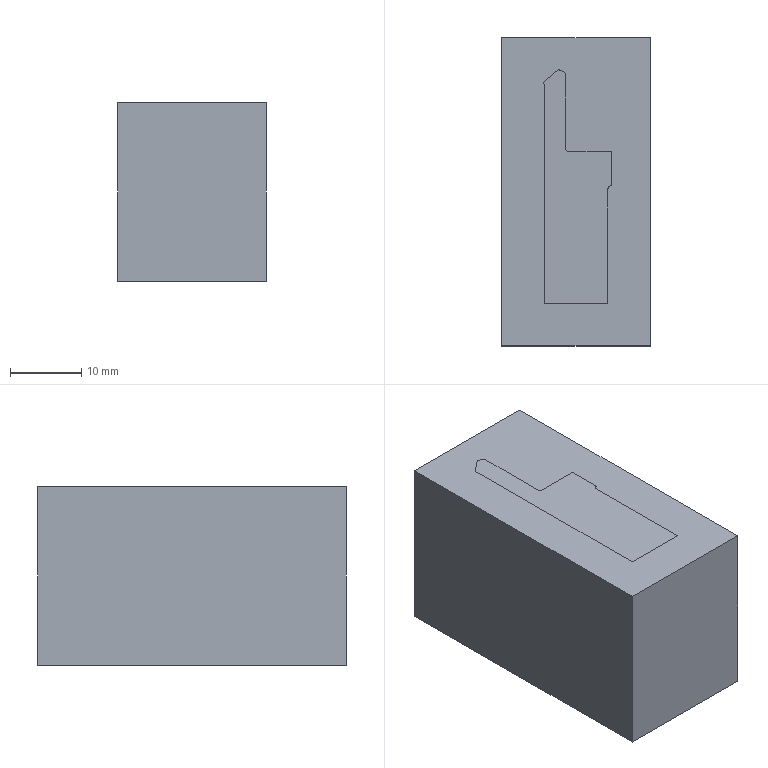Part | NX | features BREP 2 | 2 solids | 24 faces | box 20.877 x 43.224 x 25 mm | volume 39456 mm3 | plane 19 | cylinder 5 | commonest cylinder face diameters 0.9 x4 1.1 x1
STEP:
#1=CARTESIAN_POINT('',(-10.633,-22.355,-25.6));
#2=VERTEX_POINT('',#1);
#3=CARTESIAN_POINT('',(-10.633,20.868,-25.6));
#4=VERTEX_POINT('',#3);
#5=CARTESIAN_POINT('',(-10.633,-22.355,-25.6));
#6=DIRECTION('',(0.,1.,0.));
#7=VECTOR('',#6,1000.);
#8=LINE('',#5,#7);
#9=EDGE_CURVE('',#2,#4,#8,.T.);
#10=ORIENTED_EDGE('',*,*,#9,.T.);
#11=CARTESIAN_POINT('',(10.243,20.868,-25.6));
#12=VERTEX_POINT('',#11);
#13=CARTESIAN_POINT('',(-10.633,20.868,-25.6));
#14=DIRECTION('',(1.,0.,0.));
#15=VECTOR('',#14,1000.);
#16=LINE('',#13,#15);
#17=EDGE_CURVE('',#4,#12,#16,.T.);
#18=ORIENTED_EDGE('',*,*,#17,.T.);
#19=CARTESIAN_POINT('',(10.243,-22.355,-25.6));
#20=VERTEX_POINT('',#19);
#21=CARTESIAN_POINT('',(10.243,20.868,-25.6));
#22=DIRECTION('',(0.,-1.,0.));
#23=VECTOR('',#22,1000.);
#24=LINE('',#21,#23);
#25=EDGE_CURVE('',#12,#20,#24,.T.);
#26=ORIENTED_EDGE('',*,*,#25,.T.);
#27=CARTESIAN_POINT('',(10.243,-22.355,-25.6));
#28=DIRECTION('',(-1.,0.,0.));
#29=VECTOR('',#28,1000.);
#30=LINE('',#27,#29);
#31=EDGE_CURVE('',#20,#2,#30,.T.);
#32=ORIENTED_EDGE('',*,*,#31,.T.);
#33=EDGE_LOOP('',(#10,#18,#26,#32));
#34=FACE_BOUND('',#33,.T.);
#35=CARTESIAN_POINT('',(4.293,-0.3316,-25.6));
#36=VERTEX_POINT('',#35);
#37=CARTESIAN_POINT('',(4.793,0.1156,-25.6));
#38=VERTEX_POINT('',#37);
#39=CARTESIAN_POINT('',(4.743,-0.3316,-25.6));
#40=DIRECTION('',(0.,0.,-1.));
#41=DIRECTION('',(1.,0.,0.));
#42=AXIS2_PLACEMENT_3D('',#39,#40,#41);
#43=CIRCLE('',#42,0.45);
#44=EDGE_CURVE('',#36,#38,#43,.T.);
#45=ORIENTED_EDGE('',*,*,#44,.T.);
#46=CARTESIAN_POINT('',(4.793,4.918,-25.6));
#47=VERTEX_POINT('',#46);
#48=CARTESIAN_POINT('',(4.793,10.146,-25.6));
#49=DIRECTION('',(0.,1.,0.));
#50=VECTOR('',#49,1000.);
#51=LINE('',#48,#50);
#52=EDGE_CURVE('',#38,#47,#51,.T.);
#53=ORIENTED_EDGE('',*,*,#52,.T.);
#54=CARTESIAN_POINT('',(-1.233,4.918,-25.6));
#55=VERTEX_POINT('',#54);
#56=CARTESIAN_POINT('',(13.817,4.918,-25.6));
#57=DIRECTION('',(-1.,0.,0.));
#58=VECTOR('',#57,1000.);
#59=LINE('',#56,#58);
#60=EDGE_CURVE('',#47,#55,#59,.T.);
#61=ORIENTED_EDGE('',*,*,#60,.T.);
#62=CARTESIAN_POINT('',(-1.683,5.368,-25.6));
#63=VERTEX_POINT('',#62);
#64=CARTESIAN_POINT('',(-1.233,5.368,-25.6));
#65=DIRECTION('',(0.,0.,-1.));
#66=DIRECTION('',(1.,0.,0.));
#67=AXIS2_PLACEMENT_3D('',#64,#65,#66);
#68=CIRCLE('',#67,0.45);
#69=EDGE_CURVE('',#55,#63,#68,.T.);
#70=ORIENTED_EDGE('',*,*,#69,.T.);
#71=CARTESIAN_POINT('',(-1.683,15.668,-25.6));
#72=VERTEX_POINT('',#71);
#73=CARTESIAN_POINT('',(-1.683,10.146,-25.6));
#74=DIRECTION('',(0.,1.,0.));
#75=VECTOR('',#74,1000.);
#76=LINE('',#73,#75);
#77=EDGE_CURVE('',#63,#72,#76,.T.);
#78=ORIENTED_EDGE('',*,*,#77,.T.);
#79=CARTESIAN_POINT('',(-2.233,16.218,-25.6));
#80=VERTEX_POINT('',#79);
#81=CARTESIAN_POINT('',(-2.233,15.668,-25.6));
#82=DIRECTION('',(0.,0.,1.));
#83=DIRECTION('',(1.,0.,0.));
#84=AXIS2_PLACEMENT_3D('',#81,#82,#83);
#85=CIRCLE('',#84,0.55);
#86=EDGE_CURVE('',#72,#80,#85,.T.);
#87=ORIENTED_EDGE('',*,*,#86,.T.);
#88=CARTESIAN_POINT('',(-2.613,16.427,-25.6));
#89=VERTEX_POINT('',#88);
#90=CARTESIAN_POINT('',(-2.233,16.668,-25.6));
#91=DIRECTION('',(0.,0.,-1.));
#92=DIRECTION('',(1.,0.,0.));
#93=AXIS2_PLACEMENT_3D('',#90,#91,#92);
#94=CIRCLE('',#93,0.45);
#95=EDGE_CURVE('',#80,#89,#94,.T.);
#96=ORIENTED_EDGE('',*,*,#95,.T.);
#97=CARTESIAN_POINT('',(-4.816,14.657,-25.6));
#98=VERTEX_POINT('',#97);
#99=CARTESIAN_POINT('',(-5.164,14.377,-25.6));
#100=DIRECTION('',(-0.7795,-0.6264,0.));
#101=VECTOR('',#100,1000.);
#102=LINE('',#99,#101);
#103=EDGE_CURVE('',#89,#98,#102,.T.);
#104=ORIENTED_EDGE('',*,*,#103,.T.);
#105=CARTESIAN_POINT('',(-4.683,14.338,-25.6));
#106=VERTEX_POINT('',#105);
#107=CARTESIAN_POINT('',(-5.133,14.338,-25.6));
#108=DIRECTION('',(0.,0.,-1.));
#109=DIRECTION('',(1.,0.,0.));
#110=AXIS2_PLACEMENT_3D('',#107,#108,#109);
#111=CIRCLE('',#110,0.45);
#112=EDGE_CURVE('',#98,#106,#111,.T.);
#113=ORIENTED_EDGE('',*,*,#112,.T.);
#114=CARTESIAN_POINT('',(-4.683,-16.405,-25.6));
#115=VERTEX_POINT('',#114);
#116=CARTESIAN_POINT('',(-4.683,10.146,-25.6));
#117=DIRECTION('',(0.,-1.,0.));
#118=VECTOR('',#117,1000.);
#119=LINE('',#116,#118);
#120=EDGE_CURVE('',#106,#115,#119,.T.);
#121=ORIENTED_EDGE('',*,*,#120,.T.);
#122=CARTESIAN_POINT('',(4.293,-16.405,-25.6));
#123=VERTEX_POINT('',#122);
#124=CARTESIAN_POINT('',(13.817,-16.405,-25.6));
#125=DIRECTION('',(1.,0.,0.));
#126=VECTOR('',#125,1000.);
#127=LINE('',#124,#126);
#128=EDGE_CURVE('',#115,#123,#127,.T.);
#129=ORIENTED_EDGE('',*,*,#128,.T.);
#130=CARTESIAN_POINT('',(4.293,10.146,-25.6));
#131=DIRECTION('',(0.,1.,0.));
#132=VECTOR('',#131,1000.);
#133=LINE('',#130,#132);
#134=EDGE_CURVE('',#123,#36,#133,.T.);
#135=ORIENTED_EDGE('',*,*,#134,.T.);
#136=EDGE_LOOP('',(#45,#53,#61,#70,#78,#87,#96,#104,#113,#121,#129,#135));
#137=FACE_BOUND('',#136,.T.);
#138=CARTESIAN_POINT('',(0.,0.,-25.6));
#139=DIRECTION('',(0.,0.,-1.));
#140=DIRECTION('',(1.,0.,0.));
#141=AXIS2_PLACEMENT_3D('',#138,#139,#140);
#142=PLANE('',#141);
#143=ADVANCED_FACE('',(#34,#137),#142,.T.);
#144=CARTESIAN_POINT('',(-10.633,-22.355,-0.6));
#145=VERTEX_POINT('',#144);
#146=CARTESIAN_POINT('',(-10.633,20.868,-0.6));
#147=VERTEX_POINT('',#146);
#148=CARTESIAN_POINT('',(-10.633,-22.355,-0.6));
#149=DIRECTION('',(0.,1.,0.));
#150=VECTOR('',#149,1000.);
#151=LINE('',#148,#150);
#152=EDGE_CURVE('',#145,#147,#151,.T.);
#153=ORIENTED_EDGE('',*,*,#152,.F.);
#154=CARTESIAN_POINT('',(10.243,-22.355,-0.6));
#155=VERTEX_POINT('',#154);
#156=CARTESIAN_POINT('',(10.243,-22.355,-0.6));
#157=DIRECTION('',(-1.,0.,0.));
#158=VECTOR('',#157,1000.);
#159=LINE('',#156,#158);
#160=EDGE_CURVE('',#155,#145,#159,.T.);
#161=ORIENTED_EDGE('',*,*,#160,.F.);
#162=CARTESIAN_POINT('',(10.243,20.868,-0.6));
#163=VERTEX_POINT('',#162);
#164=CARTESIAN_POINT('',(10.243,20.868,-0.6));
#165=DIRECTION('',(0.,-1.,0.));
#166=VECTOR('',#165,1000.);
#167=LINE('',#164,#166);
#168=EDGE_CURVE('',#163,#155,#167,.T.);
#169=ORIENTED_EDGE('',*,*,#168,.F.);
#170=CARTESIAN_POINT('',(-10.633,20.868,-0.6));
#171=DIRECTION('',(1.,0.,0.));
#172=VECTOR('',#171,1000.);
#173=LINE('',#170,#172);
#174=EDGE_CURVE('',#147,#163,#173,.T.);
#175=ORIENTED_EDGE('',*,*,#174,.F.);
#176=EDGE_LOOP('',(#153,#161,#169,#175));
#177=FACE_BOUND('',#176,.T.);
#178=CARTESIAN_POINT('',(4.793,0.1156,-0.6));
#179=VERTEX_POINT('',#178);
#180=CARTESIAN_POINT('',(4.793,4.918,-0.6));
#181=VERTEX_POINT('',#180);
#182=CARTESIAN_POINT('',(4.793,10.146,-0.6));
#183=DIRECTION('',(0.,1.,0.));
#184=VECTOR('',#183,1000.);
#185=LINE('',#182,#184);
#186=EDGE_CURVE('',#179,#181,#185,.T.);
#187=ORIENTED_EDGE('',*,*,#186,.F.);
#188=CARTESIAN_POINT('',(4.293,-0.3316,-0.6));
#189=VERTEX_POINT('',#188);
#190=CARTESIAN_POINT('',(4.743,-0.3316,-0.6));
#191=DIRECTION('',(0.,0.,-1.));
#192=DIRECTION('',(1.,0.,0.));
#193=AXIS2_PLACEMENT_3D('',#190,#191,#192);
#194=CIRCLE('',#193,0.45);
#195=EDGE_CURVE('',#189,#179,#194,.T.);
#196=ORIENTED_EDGE('',*,*,#195,.F.);
#197=CARTESIAN_POINT('',(4.293,-16.405,-0.6));
#198=VERTEX_POINT('',#197);
#199=CARTESIAN_POINT('',(4.293,-0.3316,-0.6));
#200=DIRECTION('',(0.,1.,0.));
#201=VECTOR('',#200,1000.);
#202=LINE('',#199,#201);
#203=EDGE_CURVE('',#198,#189,#202,.T.);
#204=ORIENTED_EDGE('',*,*,#203,.F.);
#205=CARTESIAN_POINT('',(-4.683,-16.405,-0.6));
#206=VERTEX_POINT('',#205);
#207=CARTESIAN_POINT('',(-4.633,-16.405,-0.6));
#208=DIRECTION('',(1.,0.,0.));
#209=VECTOR('',#208,1000.);
#210=LINE('',#207,#209);
#211=EDGE_CURVE('',#206,#198,#210,.T.);
#212=ORIENTED_EDGE('',*,*,#211,.F.);
#213=CARTESIAN_POINT('',(-4.683,14.338,-0.6));
#214=VERTEX_POINT('',#213);
#215=CARTESIAN_POINT('',(-4.683,-17.855,-0.6));
#216=DIRECTION('',(0.,-1.,0.));
#217=VECTOR('',#216,1000.);
#218=LINE('',#215,#217);
#219=EDGE_CURVE('',#214,#206,#218,.T.);
#220=ORIENTED_EDGE('',*,*,#219,.F.);
#221=CARTESIAN_POINT('',(-4.816,14.657,-0.6));
#222=VERTEX_POINT('',#221);
#223=CARTESIAN_POINT('',(-5.133,14.338,-0.6));
#224=DIRECTION('',(0.,0.,-1.));
#225=DIRECTION('',(1.,0.,0.));
#226=AXIS2_PLACEMENT_3D('',#223,#224,#225);
#227=CIRCLE('',#226,0.45);
#228=EDGE_CURVE('',#222,#214,#227,.T.);
#229=ORIENTED_EDGE('',*,*,#228,.F.);
#230=CARTESIAN_POINT('',(-2.613,16.427,-0.6));
#231=VERTEX_POINT('',#230);
#232=CARTESIAN_POINT('',(-5.164,14.377,-0.6));
#233=DIRECTION('',(-0.7795,-0.6264,0.));
#234=VECTOR('',#233,1000.);
#235=LINE('',#232,#234);
#236=EDGE_CURVE('',#231,#222,#235,.T.);
#237=ORIENTED_EDGE('',*,*,#236,.F.);
#238=CARTESIAN_POINT('',(-2.233,16.218,-0.6));
#239=VERTEX_POINT('',#238);
#240=CARTESIAN_POINT('',(-2.233,16.668,-0.6));
#241=DIRECTION('',(0.,0.,-1.));
#242=DIRECTION('',(1.,0.,0.));
#243=AXIS2_PLACEMENT_3D('',#240,#241,#242);
#244=CIRCLE('',#243,0.45);
#245=EDGE_CURVE('',#239,#231,#244,.T.);
#246=ORIENTED_EDGE('',*,*,#245,.F.);
#247=CARTESIAN_POINT('',(-1.683,15.668,-0.6));
#248=VERTEX_POINT('',#247);
#249=CARTESIAN_POINT('',(-2.233,15.668,-0.6));
#250=DIRECTION('',(0.,0.,1.));
#251=DIRECTION('',(1.,0.,0.));
#252=AXIS2_PLACEMENT_3D('',#249,#250,#251);
#253=CIRCLE('',#252,0.55);
#254=EDGE_CURVE('',#248,#239,#253,.T.);
#255=ORIENTED_EDGE('',*,*,#254,.F.);
#256=CARTESIAN_POINT('',(-1.683,5.368,-0.6));
#257=VERTEX_POINT('',#256);
#258=CARTESIAN_POINT('',(-1.683,15.668,-0.6));
#259=DIRECTION('',(0.,1.,0.));
#260=VECTOR('',#259,1000.);
#261=LINE('',#258,#260);
#262=EDGE_CURVE('',#257,#248,#261,.T.);
#263=ORIENTED_EDGE('',*,*,#262,.F.);
#264=CARTESIAN_POINT('',(-1.233,4.918,-0.6));
#265=VERTEX_POINT('',#264);
#266=CARTESIAN_POINT('',(-1.233,5.368,-0.6));
#267=DIRECTION('',(0.,0.,-1.));
#268=DIRECTION('',(1.,0.,0.));
#269=AXIS2_PLACEMENT_3D('',#266,#267,#268);
#270=CIRCLE('',#269,0.45);
#271=EDGE_CURVE('',#265,#257,#270,.T.);
#272=ORIENTED_EDGE('',*,*,#271,.F.);
#273=CARTESIAN_POINT('',(-1.233,4.918,-0.6));
#274=DIRECTION('',(-1.,0.,0.));
#275=VECTOR('',#274,1000.);
#276=LINE('',#273,#275);
#277=EDGE_CURVE('',#181,#265,#276,.T.);
#278=ORIENTED_EDGE('',*,*,#277,.F.);
#279=EDGE_LOOP('',(#187,#196,#204,#212,#220,#229,#237,#246,#255,#263,#272,#278));
#280=FACE_BOUND('',#279,.T.);
#281=CARTESIAN_POINT('',(0.,0.,-0.6));
#282=DIRECTION('',(0.,0.,-1.));
#283=DIRECTION('',(1.,0.,0.));
#284=AXIS2_PLACEMENT_3D('',#281,#282,#283);
#285=PLANE('',#284);
#286=ADVANCED_FACE('',(#177,#280),#285,.F.);
#287=ORIENTED_EDGE('',*,*,#152,.T.);
#288=CARTESIAN_POINT('',(-10.633,20.868,-25.6));
#289=DIRECTION('',(0.,0.,1.));
#290=VECTOR('',#289,1000.);
#291=LINE('',#288,#290);
#292=EDGE_CURVE('',#4,#147,#291,.T.);
#293=ORIENTED_EDGE('',*,*,#292,.F.);
#294=ORIENTED_EDGE('',*,*,#9,.F.);
#295=CARTESIAN_POINT('',(-10.633,-22.355,-25.6));
#296=DIRECTION('',(0.,0.,1.));
#297=VECTOR('',#296,1000.);
#298=LINE('',#295,#297);
#299=EDGE_CURVE('',#2,#145,#298,.T.);
#300=ORIENTED_EDGE('',*,*,#299,.T.);
#301=EDGE_LOOP('',(#287,#293,#294,#300));
#302=FACE_BOUND('',#301,.T.);
#303=CARTESIAN_POINT('',(-10.633,-22.355,-25.6));
#304=DIRECTION('',(1.,0.,0.));
#305=DIRECTION('',(0.,-1.,0.));
#306=AXIS2_PLACEMENT_3D('',#303,#304,#305);
#307=PLANE('',#306);
#308=ADVANCED_FACE('',(#302),#307,.F.);
#309=ORIENTED_EDGE('',*,*,#174,.T.);
#310=CARTESIAN_POINT('',(10.243,20.868,-25.6));
#311=DIRECTION('',(0.,0.,1.));
#312=VECTOR('',#311,1000.);
#313=LINE('',#310,#312);
#314=EDGE_CURVE('',#12,#163,#313,.T.);
#315=ORIENTED_EDGE('',*,*,#314,.F.);
#316=ORIENTED_EDGE('',*,*,#17,.F.);
#317=ORIENTED_EDGE('',*,*,#292,.T.);
#318=EDGE_LOOP('',(#309,#315,#316,#317));
#319=FACE_BOUND('',#318,.T.);
#320=CARTESIAN_POINT('',(-10.633,20.868,-25.6));
#321=DIRECTION('',(0.,-1.,0.));
#322=DIRECTION('',(0.,0.,1.));
#323=AXIS2_PLACEMENT_3D('',#320,#321,#322);
#324=PLANE('',#323);
#325=ADVANCED_FACE('',(#319),#324,.F.);
#326=ORIENTED_EDGE('',*,*,#168,.T.);
#327=CARTESIAN_POINT('',(10.243,-22.355,-25.6));
#328=DIRECTION('',(0.,0.,1.));
#329=VECTOR('',#328,1000.);
#330=LINE('',#327,#329);
#331=EDGE_CURVE('',#20,#155,#330,.T.);
#332=ORIENTED_EDGE('',*,*,#331,.F.);
#333=ORIENTED_EDGE('',*,*,#25,.F.);
#334=ORIENTED_EDGE('',*,*,#314,.T.);
#335=EDGE_LOOP('',(#326,#332,#333,#334));
#336=FACE_BOUND('',#335,.T.);
#337=CARTESIAN_POINT('',(10.243,20.868,-25.6));
#338=DIRECTION('',(-1.,0.,0.));
#339=DIRECTION('',(0.,1.,0.));
#340=AXIS2_PLACEMENT_3D('',#337,#338,#339);
#341=PLANE('',#340);
#342=ADVANCED_FACE('',(#336),#341,.F.);
#343=ORIENTED_EDGE('',*,*,#160,.T.);
#344=ORIENTED_EDGE('',*,*,#299,.F.);
#345=ORIENTED_EDGE('',*,*,#31,.F.);
#346=ORIENTED_EDGE('',*,*,#331,.T.);
#347=EDGE_LOOP('',(#343,#344,#345,#346));
#348=FACE_BOUND('',#347,.T.);
#349=CARTESIAN_POINT('',(10.243,-22.355,-25.6));
#350=DIRECTION('',(0.,1.,0.));
#351=DIRECTION('',(1.,0.,0.));
#352=AXIS2_PLACEMENT_3D('',#349,#350,#351);
#353=PLANE('',#352);
#354=ADVANCED_FACE('',(#348),#353,.F.);
#355=CARTESIAN_POINT('',(4.293,-0.3316,0.));
#356=DIRECTION('',(0.,0.,-1.));
#357=VECTOR('',#356,1000.);
#358=LINE('',#355,#357);
#359=EDGE_CURVE('',#189,#36,#358,.T.);
#360=ORIENTED_EDGE('',*,*,#359,.T.);
#361=ORIENTED_EDGE('',*,*,#134,.F.);
#362=CARTESIAN_POINT('',(4.293,-16.405,0.));
#363=DIRECTION('',(0.,0.,-1.));
#364=VECTOR('',#363,1000.);
#365=LINE('',#362,#364);
#366=EDGE_CURVE('',#198,#123,#365,.T.);
#367=ORIENTED_EDGE('',*,*,#366,.F.);
#368=ORIENTED_EDGE('',*,*,#203,.T.);
#369=EDGE_LOOP('',(#360,#361,#367,#368));
#370=FACE_BOUND('',#369,.T.);
#371=CARTESIAN_POINT('',(4.293,-0.3316,0.));
#372=DIRECTION('',(-1.,0.,0.));
#373=DIRECTION('',(0.,1.,0.));
#374=AXIS2_PLACEMENT_3D('',#371,#372,#373);
#375=PLANE('',#374);
#376=ADVANCED_FACE('',(#370),#375,.T.);
#377=ORIENTED_EDGE('',*,*,#366,.T.);
#378=ORIENTED_EDGE('',*,*,#128,.F.);
#379=CARTESIAN_POINT('',(-4.683,-16.405,0.));
#380=DIRECTION('',(0.,0.,-1.));
#381=VECTOR('',#380,1000.);
#382=LINE('',#379,#381);
#383=EDGE_CURVE('',#206,#115,#382,.T.);
#384=ORIENTED_EDGE('',*,*,#383,.F.);
#385=ORIENTED_EDGE('',*,*,#211,.T.);
#386=EDGE_LOOP('',(#377,#378,#384,#385));
#387=FACE_BOUND('',#386,.T.);
#388=CARTESIAN_POINT('',(-4.633,-16.405,0.));
#389=DIRECTION('',(0.,-1.,0.));
#390=DIRECTION('',(-1.,0.,0.));
#391=AXIS2_PLACEMENT_3D('',#388,#389,#390);
#392=PLANE('',#391);
#393=ADVANCED_FACE('',(#387),#392,.F.);
#394=ORIENTED_EDGE('',*,*,#383,.T.);
#395=ORIENTED_EDGE('',*,*,#120,.F.);
#396=CARTESIAN_POINT('',(-4.683,14.338,0.));
#397=DIRECTION('',(0.,0.,-1.));
#398=VECTOR('',#397,1000.);
#399=LINE('',#396,#398);
#400=EDGE_CURVE('',#214,#106,#399,.T.);
#401=ORIENTED_EDGE('',*,*,#400,.F.);
#402=ORIENTED_EDGE('',*,*,#219,.T.);
#403=EDGE_LOOP('',(#394,#395,#401,#402));
#404=FACE_BOUND('',#403,.T.);
#405=CARTESIAN_POINT('',(-4.683,-17.855,0.));
#406=DIRECTION('',(1.,0.,0.));
#407=DIRECTION('',(0.,-1.,0.));
#408=AXIS2_PLACEMENT_3D('',#405,#406,#407);
#409=PLANE('',#408);
#410=ADVANCED_FACE('',(#404),#409,.T.);
#411=ORIENTED_EDGE('',*,*,#400,.T.);
#412=ORIENTED_EDGE('',*,*,#112,.F.);
#413=CARTESIAN_POINT('',(-4.816,14.657,-3.6));
#414=DIRECTION('',(0.,0.,-1.));
#415=VECTOR('',#414,1000.);
#416=LINE('',#413,#415);
#417=EDGE_CURVE('',#222,#98,#416,.T.);
#418=ORIENTED_EDGE('',*,*,#417,.F.);
#419=ORIENTED_EDGE('',*,*,#228,.T.);
#420=EDGE_LOOP('',(#411,#412,#418,#419));
#421=FACE_BOUND('',#420,.T.);
#422=CARTESIAN_POINT('',(-5.133,14.338,0.));
#423=DIRECTION('',(0.,0.,1.));
#424=DIRECTION('',(-1.,0.,0.));
#425=AXIS2_PLACEMENT_3D('',#422,#423,#424);
#426=CYLINDRICAL_SURFACE('',#425,0.45);
#427=ADVANCED_FACE('',(#421),#426,.T.);
#428=ORIENTED_EDGE('',*,*,#417,.T.);
#429=ORIENTED_EDGE('',*,*,#103,.F.);
#430=CARTESIAN_POINT('',(-2.613,16.427,-3.6));
#431=DIRECTION('',(0.,0.,-1.));
#432=VECTOR('',#431,1000.);
#433=LINE('',#430,#432);
#434=EDGE_CURVE('',#231,#89,#433,.T.);
#435=ORIENTED_EDGE('',*,*,#434,.F.);
#436=ORIENTED_EDGE('',*,*,#236,.T.);
#437=EDGE_LOOP('',(#428,#429,#435,#436));
#438=FACE_BOUND('',#437,.T.);
#439=CARTESIAN_POINT('',(-5.164,14.377,0.));
#440=DIRECTION('',(0.6264,-0.7795,0.));
#441=DIRECTION('',(-0.7795,-0.6264,0.));
#442=AXIS2_PLACEMENT_3D('',#439,#440,#441);
#443=PLANE('',#442);
#444=ADVANCED_FACE('',(#438),#443,.T.);
#445=ORIENTED_EDGE('',*,*,#434,.T.);
#446=ORIENTED_EDGE('',*,*,#95,.F.);
#447=CARTESIAN_POINT('',(-2.233,16.218,0.));
#448=DIRECTION('',(0.,0.,-1.));
#449=VECTOR('',#448,1000.);
#450=LINE('',#447,#449);
#451=EDGE_CURVE('',#239,#80,#450,.T.);
#452=ORIENTED_EDGE('',*,*,#451,.F.);
#453=ORIENTED_EDGE('',*,*,#245,.T.);
#454=EDGE_LOOP('',(#445,#446,#452,#453));
#455=FACE_BOUND('',#454,.T.);
#456=CARTESIAN_POINT('',(-2.233,16.668,0.));
#457=DIRECTION('',(0.,0.,1.));
#458=DIRECTION('',(-1.,0.,0.));
#459=AXIS2_PLACEMENT_3D('',#456,#457,#458);
#460=CYLINDRICAL_SURFACE('',#459,0.45);
#461=ADVANCED_FACE('',(#455),#460,.T.);
#462=ORIENTED_EDGE('',*,*,#451,.T.);
#463=ORIENTED_EDGE('',*,*,#86,.F.);
#464=CARTESIAN_POINT('',(-1.683,15.668,0.));
#465=DIRECTION('',(0.,0.,-1.));
#466=VECTOR('',#465,1000.);
#467=LINE('',#464,#466);
#468=EDGE_CURVE('',#248,#72,#467,.T.);
#469=ORIENTED_EDGE('',*,*,#468,.F.);
#470=ORIENTED_EDGE('',*,*,#254,.T.);
#471=EDGE_LOOP('',(#462,#463,#469,#470));
#472=FACE_BOUND('',#471,.T.);
#473=CARTESIAN_POINT('',(-2.233,15.668,0.));
#474=DIRECTION('',(0.,0.,1.));
#475=DIRECTION('',(-1.,0.,0.));
#476=AXIS2_PLACEMENT_3D('',#473,#474,#475);
#477=CYLINDRICAL_SURFACE('',#476,0.55);
#478=ADVANCED_FACE('',(#472),#477,.F.);
#479=ORIENTED_EDGE('',*,*,#468,.T.);
#480=ORIENTED_EDGE('',*,*,#77,.F.);
#481=CARTESIAN_POINT('',(-1.683,5.368,0.));
#482=DIRECTION('',(0.,0.,-1.));
#483=VECTOR('',#482,1000.);
#484=LINE('',#481,#483);
#485=EDGE_CURVE('',#257,#63,#484,.T.);
#486=ORIENTED_EDGE('',*,*,#485,.F.);
#487=ORIENTED_EDGE('',*,*,#262,.T.);
#488=EDGE_LOOP('',(#479,#480,#486,#487));
#489=FACE_BOUND('',#488,.T.);
#490=CARTESIAN_POINT('',(-1.683,15.668,0.));
#491=DIRECTION('',(-1.,0.,0.));
#492=DIRECTION('',(0.,1.,0.));
#493=AXIS2_PLACEMENT_3D('',#490,#491,#492);
#494=PLANE('',#493);
#495=ADVANCED_FACE('',(#489),#494,.T.);
#496=ORIENTED_EDGE('',*,*,#485,.T.);
#497=ORIENTED_EDGE('',*,*,#69,.F.);
#498=CARTESIAN_POINT('',(-1.233,4.918,0.));
#499=DIRECTION('',(0.,0.,-1.));
#500=VECTOR('',#499,1000.);
#501=LINE('',#498,#500);
#502=EDGE_CURVE('',#265,#55,#501,.T.);
#503=ORIENTED_EDGE('',*,*,#502,.F.);
#504=ORIENTED_EDGE('',*,*,#271,.T.);
#505=EDGE_LOOP('',(#496,#497,#503,#504));
#506=FACE_BOUND('',#505,.T.);
#507=CARTESIAN_POINT('',(-1.233,5.368,0.));
#508=DIRECTION('',(0.,0.,1.));
#509=DIRECTION('',(-1.,0.,0.));
#510=AXIS2_PLACEMENT_3D('',#507,#508,#509);
#511=CYLINDRICAL_SURFACE('',#510,0.45);
#512=ADVANCED_FACE('',(#506),#511,.T.);
#513=ORIENTED_EDGE('',*,*,#502,.T.);
#514=ORIENTED_EDGE('',*,*,#60,.F.);
#515=CARTESIAN_POINT('',(4.793,4.918,0.));
#516=DIRECTION('',(0.,0.,-1.));
#517=VECTOR('',#516,1000.);
#518=LINE('',#515,#517);
#519=EDGE_CURVE('',#181,#47,#518,.T.);
#520=ORIENTED_EDGE('',*,*,#519,.F.);
#521=ORIENTED_EDGE('',*,*,#277,.T.);
#522=EDGE_LOOP('',(#513,#514,#520,#521));
#523=FACE_BOUND('',#522,.T.);
#524=CARTESIAN_POINT('',(-1.233,4.918,0.));
#525=DIRECTION('',(0.,-1.,0.));
#526=DIRECTION('',(-1.,0.,0.));
#527=AXIS2_PLACEMENT_3D('',#524,#525,#526);
#528=PLANE('',#527);
#529=ADVANCED_FACE('',(#523),#528,.T.);
#530=ORIENTED_EDGE('',*,*,#519,.T.);
#531=ORIENTED_EDGE('',*,*,#52,.F.);
#532=CARTESIAN_POINT('',(4.793,0.1156,-3.6));
#533=DIRECTION('',(0.,0.,-1.));
#534=VECTOR('',#533,1000.);
#535=LINE('',#532,#534);
#536=EDGE_CURVE('',#179,#38,#535,.T.);
#537=ORIENTED_EDGE('',*,*,#536,.F.);
#538=ORIENTED_EDGE('',*,*,#186,.T.);
#539=EDGE_LOOP('',(#530,#531,#537,#538));
#540=FACE_BOUND('',#539,.T.);
#541=CARTESIAN_POINT('',(4.793,10.146,0.));
#542=DIRECTION('',(-1.,0.,0.));
#543=DIRECTION('',(0.,1.,0.));
#544=AXIS2_PLACEMENT_3D('',#541,#542,#543);
#545=PLANE('',#544);
#546=ADVANCED_FACE('',(#540),#545,.T.);
#547=ORIENTED_EDGE('',*,*,#536,.T.);
#548=ORIENTED_EDGE('',*,*,#44,.F.);
#549=ORIENTED_EDGE('',*,*,#359,.F.);
#550=ORIENTED_EDGE('',*,*,#195,.T.);
#551=EDGE_LOOP('',(#547,#548,#549,#550));
#552=FACE_BOUND('',#551,.T.);
#553=CARTESIAN_POINT('',(4.743,-0.3316,0.));
#554=DIRECTION('',(0.,0.,1.));
#555=DIRECTION('',(-1.,0.,0.));
#556=AXIS2_PLACEMENT_3D('',#553,#554,#555);
#557=CYLINDRICAL_SURFACE('',#556,0.45);
#558=ADVANCED_FACE('',(#552),#557,.T.);
#559=CLOSED_SHELL('',(#143,#286,#308,#325,#342,#354,#376,#393,#410,#427,#444,#461,#478,#495,#512,#529,#546,#558));
#560=MANIFOLD_SOLID_BREP('',#559);
#561=CARTESIAN_POINT('',(-10.633,-22.355,-0.6));
#562=VERTEX_POINT('',#561);
#563=CARTESIAN_POINT('',(-10.633,20.868,-0.6));
#564=VERTEX_POINT('',#563);
#565=CARTESIAN_POINT('',(-10.633,-22.355,-0.6));
#566=DIRECTION('',(0.,1.,0.));
#567=VECTOR('',#566,1000.);
#568=LINE('',#565,#567);
#569=EDGE_CURVE('',#562,#564,#568,.T.);
#570=ORIENTED_EDGE('',*,*,#569,.T.);
#571=CARTESIAN_POINT('',(-10.633,20.868,-25.6));
#572=VERTEX_POINT('',#571);
#573=CARTESIAN_POINT('',(-10.633,20.868,-25.6));
#574=DIRECTION('',(0.,0.,1.));
#575=VECTOR('',#574,1000.);
#576=LINE('',#573,#575);
#577=EDGE_CURVE('',#572,#564,#576,.T.);
#578=ORIENTED_EDGE('',*,*,#577,.F.);
#579=CARTESIAN_POINT('',(-10.633,-22.355,-25.6));
#580=VERTEX_POINT('',#579);
#581=CARTESIAN_POINT('',(-10.633,-22.355,-25.6));
#582=DIRECTION('',(0.,1.,0.));
#583=VECTOR('',#582,1000.);
#584=LINE('',#581,#583);
#585=EDGE_CURVE('',#580,#572,#584,.T.);
#586=ORIENTED_EDGE('',*,*,#585,.F.);
#587=CARTESIAN_POINT('',(-10.633,-22.355,-25.6));
#588=DIRECTION('',(0.,0.,1.));
#589=VECTOR('',#588,1000.);
#590=LINE('',#587,#589);
#591=EDGE_CURVE('',#580,#562,#590,.T.);
#592=ORIENTED_EDGE('',*,*,#591,.T.);
#593=EDGE_LOOP('',(#570,#578,#586,#592));
#594=FACE_BOUND('',#593,.T.);
#595=CARTESIAN_POINT('',(-10.633,-22.355,-25.6));
#596=DIRECTION('',(1.,0.,0.));
#597=DIRECTION('',(0.,-1.,0.));
#598=AXIS2_PLACEMENT_3D('',#595,#596,#597);
#599=PLANE('',#598);
#600=ADVANCED_FACE('',(#594),#599,.F.);
#601=CARTESIAN_POINT('',(10.243,20.868,-0.6));
#602=VERTEX_POINT('',#601);
#603=CARTESIAN_POINT('',(-10.633,20.868,-0.6));
#604=DIRECTION('',(1.,0.,0.));
#605=VECTOR('',#604,1000.);
#606=LINE('',#603,#605);
#607=EDGE_CURVE('',#564,#602,#606,.T.);
#608=ORIENTED_EDGE('',*,*,#607,.T.);
#609=CARTESIAN_POINT('',(10.243,20.868,-25.6));
#610=VERTEX_POINT('',#609);
#611=CARTESIAN_POINT('',(10.243,20.868,-25.6));
#612=DIRECTION('',(0.,0.,1.));
#613=VECTOR('',#612,1000.);
#614=LINE('',#611,#613);
#615=EDGE_CURVE('',#610,#602,#614,.T.);
#616=ORIENTED_EDGE('',*,*,#615,.F.);
#617=CARTESIAN_POINT('',(-10.633,20.868,-25.6));
#618=DIRECTION('',(1.,0.,0.));
#619=VECTOR('',#618,1000.);
#620=LINE('',#617,#619);
#621=EDGE_CURVE('',#572,#610,#620,.T.);
#622=ORIENTED_EDGE('',*,*,#621,.F.);
#623=ORIENTED_EDGE('',*,*,#577,.T.);
#624=EDGE_LOOP('',(#608,#616,#622,#623));
#625=FACE_BOUND('',#624,.T.);
#626=CARTESIAN_POINT('',(-10.633,20.868,-25.6));
#627=DIRECTION('',(0.,-1.,0.));
#628=DIRECTION('',(0.,0.,1.));
#629=AXIS2_PLACEMENT_3D('',#626,#627,#628);
#630=PLANE('',#629);
#631=ADVANCED_FACE('',(#625),#630,.F.);
#632=CARTESIAN_POINT('',(10.243,-22.355,-0.6));
#633=VERTEX_POINT('',#632);
#634=CARTESIAN_POINT('',(10.243,20.868,-0.6));
#635=DIRECTION('',(0.,-1.,0.));
#636=VECTOR('',#635,1000.);
#637=LINE('',#634,#636);
#638=EDGE_CURVE('',#602,#633,#637,.T.);
#639=ORIENTED_EDGE('',*,*,#638,.T.);
#640=CARTESIAN_POINT('',(10.243,-22.355,-25.6));
#641=VERTEX_POINT('',#640);
#642=CARTESIAN_POINT('',(10.243,-22.355,-25.6));
#643=DIRECTION('',(0.,0.,1.));
#644=VECTOR('',#643,1000.);
#645=LINE('',#642,#644);
#646=EDGE_CURVE('',#641,#633,#645,.T.);
#647=ORIENTED_EDGE('',*,*,#646,.F.);
#648=CARTESIAN_POINT('',(10.243,20.868,-25.6));
#649=DIRECTION('',(0.,-1.,0.));
#650=VECTOR('',#649,1000.);
#651=LINE('',#648,#650);
#652=EDGE_CURVE('',#610,#641,#651,.T.);
#653=ORIENTED_EDGE('',*,*,#652,.F.);
#654=ORIENTED_EDGE('',*,*,#615,.T.);
#655=EDGE_LOOP('',(#639,#647,#653,#654));
#656=FACE_BOUND('',#655,.T.);
#657=CARTESIAN_POINT('',(10.243,20.868,-25.6));
#658=DIRECTION('',(-1.,0.,0.));
#659=DIRECTION('',(0.,1.,0.));
#660=AXIS2_PLACEMENT_3D('',#657,#658,#659);
#661=PLANE('',#660);
#662=ADVANCED_FACE('',(#656),#661,.F.);
#663=CARTESIAN_POINT('',(10.243,-22.355,-0.6));
#664=DIRECTION('',(-1.,0.,0.));
#665=VECTOR('',#664,1000.);
#666=LINE('',#663,#665);
#667=EDGE_CURVE('',#633,#562,#666,.T.);
#668=ORIENTED_EDGE('',*,*,#667,.T.);
#669=ORIENTED_EDGE('',*,*,#591,.F.);
#670=CARTESIAN_POINT('',(10.243,-22.355,-25.6));
#671=DIRECTION('',(-1.,0.,0.));
#672=VECTOR('',#671,1000.);
#673=LINE('',#670,#672);
#674=EDGE_CURVE('',#641,#580,#673,.T.);
#675=ORIENTED_EDGE('',*,*,#674,.F.);
#676=ORIENTED_EDGE('',*,*,#646,.T.);
#677=EDGE_LOOP('',(#668,#669,#675,#676));
#678=FACE_BOUND('',#677,.T.);
#679=CARTESIAN_POINT('',(10.243,-22.355,-25.6));
#680=DIRECTION('',(0.,1.,0.));
#681=DIRECTION('',(1.,0.,0.));
#682=AXIS2_PLACEMENT_3D('',#679,#680,#681);
#683=PLANE('',#682);
#684=ADVANCED_FACE('',(#678),#683,.F.);
#685=ORIENTED_EDGE('',*,*,#585,.T.);
#686=ORIENTED_EDGE('',*,*,#621,.T.);
#687=ORIENTED_EDGE('',*,*,#652,.T.);
#688=ORIENTED_EDGE('',*,*,#674,.T.);
#689=EDGE_LOOP('',(#685,#686,#687,#688));
#690=FACE_BOUND('',#689,.T.);
#691=CARTESIAN_POINT('',(0.,0.,-25.6));
#692=DIRECTION('',(0.,0.,-1.));
#693=DIRECTION('',(1.,0.,0.));
#694=AXIS2_PLACEMENT_3D('',#691,#692,#693);
#695=PLANE('',#694);
#696=ADVANCED_FACE('',(#690),#695,.T.);
#697=ORIENTED_EDGE('',*,*,#569,.F.);
#698=ORIENTED_EDGE('',*,*,#667,.F.);
#699=ORIENTED_EDGE('',*,*,#638,.F.);
#700=ORIENTED_EDGE('',*,*,#607,.F.);
#701=EDGE_LOOP('',(#697,#698,#699,#700));
#702=FACE_BOUND('',#701,.T.);
#703=CARTESIAN_POINT('',(0.,0.,-0.6));
#704=DIRECTION('',(0.,0.,-1.));
#705=DIRECTION('',(1.,0.,0.));
#706=AXIS2_PLACEMENT_3D('',#703,#704,#705);
#707=PLANE('',#706);
#708=ADVANCED_FACE('',(#702),#707,.F.);
#709=CLOSED_SHELL('',(#600,#631,#662,#684,#696,#708));
#710=MANIFOLD_SOLID_BREP('',#709);
#711=(LENGTH_UNIT()NAMED_UNIT(*)SI_UNIT(.MILLI.,.METRE.));
#712=UNCERTAINTY_MEASURE_WITH_UNIT(LENGTH_MEASURE(0.00001),#711,'','');
#713=(NAMED_UNIT(*)PLANE_ANGLE_UNIT()SI_UNIT($,.RADIAN.));
#714=(NAMED_UNIT(*)SI_UNIT($,.STERADIAN.)SOLID_ANGLE_UNIT());
#715=(GEOMETRIC_REPRESENTATION_CONTEXT(3)GLOBAL_UNCERTAINTY_ASSIGNED_CONTEXT((#712))GLOBAL_UNIT_ASSIGNED_CONTEXT((#711,#713,#714))REPRESENTATION_CONTEXT('',''));
#716=ADVANCED_BREP_SHAPE_REPRESENTATION('',(#560,#710),#715);